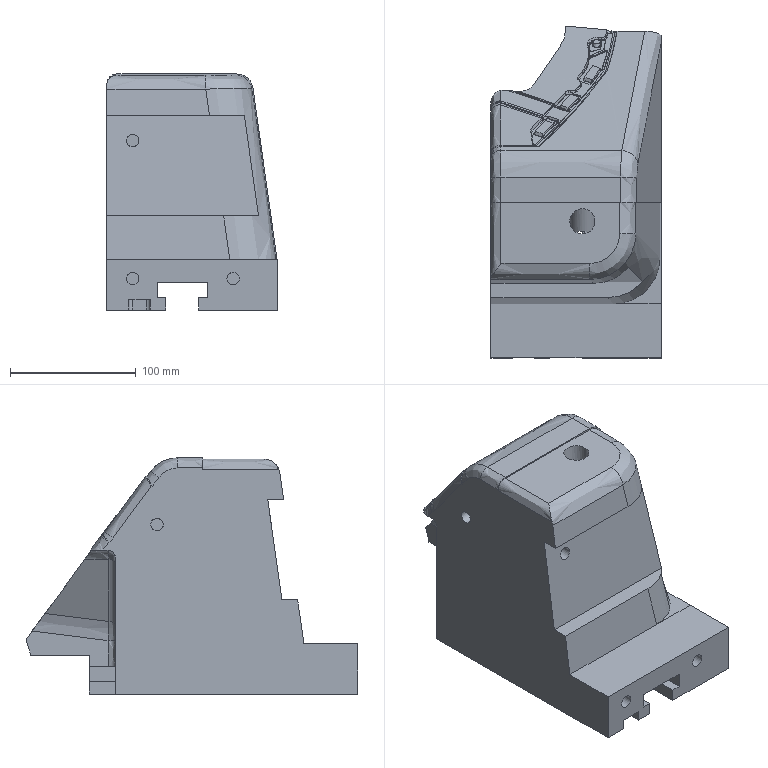Part | STEP file | solid 23 | 1 solid | 330 faces | box 135.51 x 264.332 x 188.118 mm | volume 3455186 mm3 | spline 238 | plane 48 | cylinder 34 | sphere 8 | other 2 | commonest cylinder face diameters 10 x17 1.013 x3 1.621 x3 6 x2 10.13 x2 0.405 x1